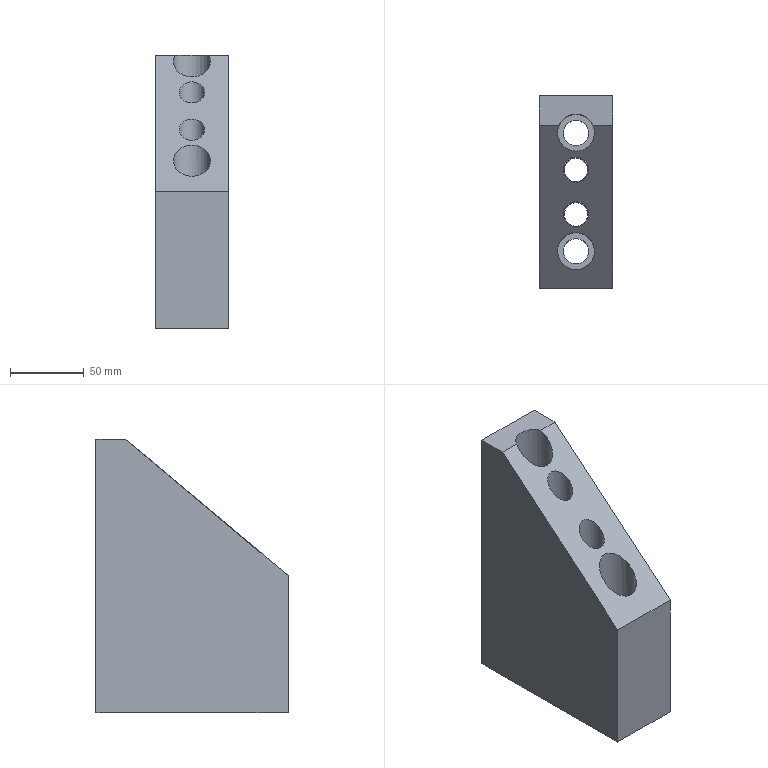Part | NX | features solid 2 | 1 solid | 19 faces | box 50 x 130 x 185 mm | volume 754988 mm3 | plane 11 | cylinder 8 | commonest cylinder face diameters 17 x4 16 x2 25 x2
STEP:
#1=CARTESIAN_POINT('',(-210.,-307.5,5.));
#2=VERTEX_POINT('',#1);
#3=CARTESIAN_POINT('',(-210.,-307.5,-150.));
#4=VERTEX_POINT('',#3);
#5=CARTESIAN_POINT('',(-210.,-307.5,-150.));
#6=DIRECTION('',(0.,0.,1.));
#7=VECTOR('',#6,1000.);
#8=LINE('',#5,#7);
#9=EDGE_CURVE('',#2,#4,#8,.F.);
#10=ORIENTED_EDGE('',*,*,#9,.T.);
#11=ORIENTED_EDGE('',*,*,#9,.F.);
#12=CARTESIAN_POINT('',(-210.,-295.,5.));
#13=VERTEX_POINT('',#12);
#14=CARTESIAN_POINT('',(-210.,-295.,5.));
#15=DIRECTION('',(0.,1.,0.));
#16=VECTOR('',#15,1000.);
#17=LINE('',#14,#16);
#18=EDGE_CURVE('',#13,#2,#17,.F.);
#19=ORIENTED_EDGE('',*,*,#18,.F.);
#20=CARTESIAN_POINT('',(-210.,-295.,-180.));
#21=VERTEX_POINT('',#20);
#22=CARTESIAN_POINT('',(-210.,-295.,5.));
#23=DIRECTION('',(0.,0.,1.));
#24=VECTOR('',#23,1000.);
#25=LINE('',#22,#24);
#26=EDGE_CURVE('',#13,#21,#25,.F.);
#27=ORIENTED_EDGE('',*,*,#26,.T.);
#28=CARTESIAN_POINT('',(-210.,-303.5,-180.));
#29=VERTEX_POINT('',#28);
#30=CARTESIAN_POINT('',(-210.,-275.,-180.));
#31=DIRECTION('',(0.,1.,0.));
#32=VECTOR('',#31,1000.);
#33=LINE('',#30,#32);
#34=EDGE_CURVE('',#29,#21,#33,.T.);
#35=ORIENTED_EDGE('',*,*,#34,.F.);
#36=CARTESIAN_POINT('',(-210.,-303.5,-150.));
#37=VERTEX_POINT('',#36);
#38=CARTESIAN_POINT('',(-210.,-303.5,-210.));
#39=DIRECTION('',(0.,0.,1.));
#40=VECTOR('',#39,1000.);
#41=LINE('',#38,#40);
#42=EDGE_CURVE('',#37,#29,#41,.F.);
#43=ORIENTED_EDGE('',*,*,#42,.F.);
#44=ORIENTED_EDGE('',*,*,#42,.T.);
#45=CARTESIAN_POINT('',(-210.,-425.,-180.));
#46=VERTEX_POINT('',#45);
#47=CARTESIAN_POINT('',(-210.,-275.,-180.));
#48=DIRECTION('',(0.,1.,0.));
#49=VECTOR('',#48,1000.);
#50=LINE('',#47,#49);
#51=EDGE_CURVE('',#46,#29,#50,.T.);
#52=ORIENTED_EDGE('',*,*,#51,.F.);
#53=CARTESIAN_POINT('',(-210.,-425.,-87.301));
#54=VERTEX_POINT('',#53);
#55=CARTESIAN_POINT('',(-210.,-425.,-120.405));
#56=DIRECTION('',(0.,0.,1.));
#57=VECTOR('',#56,1000.);
#58=LINE('',#55,#57);
#59=EDGE_CURVE('',#46,#54,#58,.T.);
#60=ORIENTED_EDGE('',*,*,#59,.T.);
#61=CARTESIAN_POINT('',(-210.,-315.,5.));
#62=VERTEX_POINT('',#61);
#63=CARTESIAN_POINT('',(-210.,-291.527,24.696));
#64=DIRECTION('',(0.,0.766,0.6428));
#65=VECTOR('',#64,1000.);
#66=LINE('',#63,#65);
#67=EDGE_CURVE('',#62,#54,#66,.F.);
#68=ORIENTED_EDGE('',*,*,#67,.F.);
#69=CARTESIAN_POINT('',(-210.,-275.,5.));
#70=DIRECTION('',(0.,-1.,0.));
#71=VECTOR('',#70,1000.);
#72=LINE('',#69,#71);
#73=EDGE_CURVE('',#2,#62,#72,.T.);
#74=ORIENTED_EDGE('',*,*,#73,.F.);
#75=EDGE_LOOP('',(#10,#11,#19,#27,#35,#43,#44,#52,#60,#68,#74));
#76=FACE_BOUND('',#75,.T.);
#77=CARTESIAN_POINT('',(-210.,-275.,5.));
#78=DIRECTION('',(-1.,0.,0.));
#79=DIRECTION('',(0.,0.,-1.));
#80=AXIS2_PLACEMENT_3D('',#77,#78,#79);
#81=PLANE('',#80);
#82=ADVANCED_FACE('',(#76),#81,.T.);
#83=CARTESIAN_POINT('',(-193.,-375.,-180.));
#84=VERTEX_POINT('',#83);
#85=CARTESIAN_POINT('',(-185.,-375.,-180.));
#86=DIRECTION('',(0.,0.,-1.));
#87=DIRECTION('',(-1.,0.,0.));
#88=AXIS2_PLACEMENT_3D('',#85,#86,#87);
#89=CIRCLE('',#88,8.);
#90=EDGE_CURVE('',#84,#84,#89,.F.);
#91=ORIENTED_EDGE('',*,*,#90,.T.);
#92=EDGE_LOOP('',(#91));
#93=FACE_BOUND('',#92,.T.);
#94=CARTESIAN_POINT('',(-193.,-345.,-180.));
#95=VERTEX_POINT('',#94);
#96=CARTESIAN_POINT('',(-185.,-345.,-180.));
#97=DIRECTION('',(0.,0.,-1.));
#98=DIRECTION('',(-1.,0.,0.));
#99=AXIS2_PLACEMENT_3D('',#96,#97,#98);
#100=CIRCLE('',#99,8.);
#101=EDGE_CURVE('',#95,#95,#100,.F.);
#102=ORIENTED_EDGE('',*,*,#101,.T.);
#103=EDGE_LOOP('',(#102));
#104=FACE_BOUND('',#103,.T.);
#105=CARTESIAN_POINT('',(-193.5,-400.,-180.));
#106=VERTEX_POINT('',#105);
#107=CARTESIAN_POINT('',(-185.,-400.,-180.));
#108=DIRECTION('',(0.,0.,-1.));
#109=DIRECTION('',(-1.,0.,0.));
#110=AXIS2_PLACEMENT_3D('',#107,#108,#109);
#111=CIRCLE('',#110,8.5);
#112=EDGE_CURVE('',#106,#106,#111,.F.);
#113=ORIENTED_EDGE('',*,*,#112,.T.);
#114=EDGE_LOOP('',(#113));
#115=FACE_BOUND('',#114,.T.);
#116=CARTESIAN_POINT('',(-193.5,-320.,-180.));
#117=VERTEX_POINT('',#116);
#118=CARTESIAN_POINT('',(-185.,-320.,-180.));
#119=DIRECTION('',(0.,0.,-1.));
#120=DIRECTION('',(-1.,0.,0.));
#121=AXIS2_PLACEMENT_3D('',#118,#119,#120);
#122=CIRCLE('',#121,8.5);
#123=EDGE_CURVE('',#117,#117,#122,.F.);
#124=ORIENTED_EDGE('',*,*,#123,.T.);
#125=EDGE_LOOP('',(#124));
#126=FACE_BOUND('',#125,.T.);
#127=ORIENTED_EDGE('',*,*,#51,.T.);
#128=ORIENTED_EDGE('',*,*,#34,.T.);
#129=CARTESIAN_POINT('',(-160.,-295.,-180.));
#130=VERTEX_POINT('',#129);
#131=CARTESIAN_POINT('',(-205.,-295.,-180.));
#132=DIRECTION('',(1.,0.,0.));
#133=VECTOR('',#132,1000.);
#134=LINE('',#131,#133);
#135=EDGE_CURVE('',#130,#21,#134,.F.);
#136=ORIENTED_EDGE('',*,*,#135,.F.);
#137=CARTESIAN_POINT('',(-160.,-425.,-180.));
#138=VERTEX_POINT('',#137);
#139=CARTESIAN_POINT('',(-160.,-275.,-180.));
#140=DIRECTION('',(0.,-1.,0.));
#141=VECTOR('',#140,1000.);
#142=LINE('',#139,#141);
#143=EDGE_CURVE('',#138,#130,#142,.F.);
#144=ORIENTED_EDGE('',*,*,#143,.F.);
#145=CARTESIAN_POINT('',(-205.,-425.,-180.));
#146=DIRECTION('',(-1.,0.,0.));
#147=VECTOR('',#146,1000.);
#148=LINE('',#145,#147);
#149=EDGE_CURVE('',#138,#46,#148,.T.);
#150=ORIENTED_EDGE('',*,*,#149,.T.);
#151=EDGE_LOOP('',(#127,#128,#136,#144,#150));
#152=FACE_BOUND('',#151,.T.);
#153=CARTESIAN_POINT('',(-205.,-275.,-180.));
#154=DIRECTION('',(0.,0.,-1.));
#155=DIRECTION('',(1.,0.,0.));
#156=AXIS2_PLACEMENT_3D('',#153,#154,#155);
#157=PLANE('',#156);
#158=ADVANCED_FACE('',(#93,#104,#115,#126,#152),#157,.T.);
#159=CARTESIAN_POINT('',(-160.,-295.,5.));
#160=VERTEX_POINT('',#159);
#161=CARTESIAN_POINT('',(-160.,-295.,5.));
#162=DIRECTION('',(0.,0.,-1.));
#163=VECTOR('',#162,1000.);
#164=LINE('',#161,#163);
#165=EDGE_CURVE('',#160,#130,#164,.T.);
#166=ORIENTED_EDGE('',*,*,#165,.F.);
#167=CARTESIAN_POINT('',(-160.,-315.,5.));
#168=VERTEX_POINT('',#167);
#169=CARTESIAN_POINT('',(-160.,-295.,5.));
#170=DIRECTION('',(0.,1.,0.));
#171=VECTOR('',#170,1000.);
#172=LINE('',#169,#171);
#173=EDGE_CURVE('',#168,#160,#172,.T.);
#174=ORIENTED_EDGE('',*,*,#173,.F.);
#175=CARTESIAN_POINT('',(-160.,-425.,-87.301));
#176=VERTEX_POINT('',#175);
#177=CARTESIAN_POINT('',(-160.,-330.716,-8.188));
#178=DIRECTION('',(0.,-0.766,-0.6428));
#179=VECTOR('',#178,1000.);
#180=LINE('',#177,#179);
#181=EDGE_CURVE('',#168,#176,#180,.T.);
#182=ORIENTED_EDGE('',*,*,#181,.T.);
#183=CARTESIAN_POINT('',(-160.,-425.,-120.405));
#184=DIRECTION('',(0.,0.,1.));
#185=VECTOR('',#184,1000.);
#186=LINE('',#183,#185);
#187=EDGE_CURVE('',#176,#138,#186,.F.);
#188=ORIENTED_EDGE('',*,*,#187,.T.);
#189=ORIENTED_EDGE('',*,*,#143,.T.);
#190=EDGE_LOOP('',(#166,#174,#182,#188,#189));
#191=FACE_BOUND('',#190,.T.);
#192=CARTESIAN_POINT('',(-160.,-275.,5.));
#193=DIRECTION('',(-1.,0.,0.));
#194=DIRECTION('',(0.,0.,-1.));
#195=AXIS2_PLACEMENT_3D('',#192,#193,#194);
#196=PLANE('',#195);
#197=ADVANCED_FACE('',(#191),#196,.F.);
#198=CARTESIAN_POINT('',(-196.456,-315.,5.));
#199=VERTEX_POINT('',#198);
#200=CARTESIAN_POINT('',(-205.,-315.,5.));
#201=DIRECTION('',(1.,0.,0.));
#202=VECTOR('',#201,1000.);
#203=LINE('',#200,#202);
#204=EDGE_CURVE('',#62,#199,#203,.T.);
#205=ORIENTED_EDGE('',*,*,#204,.T.);
#206=CARTESIAN_POINT('',(-173.544,-315.,5.));
#207=VERTEX_POINT('',#206);
#208=CARTESIAN_POINT('',(-185.,-320.,5.));
#209=DIRECTION('',(0.,0.,-1.));
#210=DIRECTION('',(-1.,0.,0.));
#211=AXIS2_PLACEMENT_3D('',#208,#209,#210);
#212=CIRCLE('',#211,12.5);
#213=EDGE_CURVE('',#199,#207,#212,.T.);
#214=ORIENTED_EDGE('',*,*,#213,.T.);
#215=CARTESIAN_POINT('',(-205.,-315.,5.));
#216=DIRECTION('',(1.,0.,0.));
#217=VECTOR('',#216,1000.);
#218=LINE('',#215,#217);
#219=EDGE_CURVE('',#207,#168,#218,.T.);
#220=ORIENTED_EDGE('',*,*,#219,.T.);
#221=ORIENTED_EDGE('',*,*,#173,.T.);
#222=CARTESIAN_POINT('',(-110.,-295.,5.));
#223=DIRECTION('',(1.,0.,0.));
#224=VECTOR('',#223,1000.);
#225=LINE('',#222,#224);
#226=EDGE_CURVE('',#13,#160,#225,.T.);
#227=ORIENTED_EDGE('',*,*,#226,.F.);
#228=ORIENTED_EDGE('',*,*,#18,.T.);
#229=ORIENTED_EDGE('',*,*,#73,.T.);
#230=EDGE_LOOP('',(#205,#214,#220,#221,#227,#228,#229));
#231=FACE_BOUND('',#230,.T.);
#232=CARTESIAN_POINT('',(-110.,-295.,5.));
#233=DIRECTION('',(0.,0.,-1.));
#234=DIRECTION('',(-1.,0.,0.));
#235=AXIS2_PLACEMENT_3D('',#232,#233,#234);
#236=PLANE('',#235);
#237=ADVANCED_FACE('',(#231),#236,.F.);
#238=CARTESIAN_POINT('',(-185.,-366.5,-38.214));
#239=VERTEX_POINT('',#238);
#240=CARTESIAN_POINT('',(-185.,-375.,-45.346));
#241=DIRECTION('',(0.,-0.6428,0.766));
#242=DIRECTION('',(0.,0.766,0.6428));
#243=AXIS2_PLACEMENT_3D('',#240,#241,#242);
#244=ELLIPSE('',#243,11.096,8.5);
#245=EDGE_CURVE('',#239,#239,#244,.T.);
#246=ORIENTED_EDGE('',*,*,#245,.F.);
#247=EDGE_LOOP('',(#246));
#248=FACE_BOUND('',#247,.T.);
#249=CARTESIAN_POINT('',(-185.,-336.5,-13.041));
#250=VERTEX_POINT('',#249);
#251=CARTESIAN_POINT('',(-185.,-345.,-20.173));
#252=DIRECTION('',(0.,-0.6428,0.766));
#253=DIRECTION('',(0.,0.766,0.6428));
#254=AXIS2_PLACEMENT_3D('',#251,#252,#253);
#255=ELLIPSE('',#254,11.096,8.5);
#256=EDGE_CURVE('',#250,#250,#255,.T.);
#257=ORIENTED_EDGE('',*,*,#256,.F.);
#258=EDGE_LOOP('',(#257));
#259=FACE_BOUND('',#258,.T.);
#260=CARTESIAN_POINT('',(-185.,-387.5,-55.835));
#261=VERTEX_POINT('',#260);
#262=CARTESIAN_POINT('',(-185.,-400.,-66.323));
#263=DIRECTION('',(0.,-0.6428,0.766));
#264=DIRECTION('',(0.,0.766,0.6428));
#265=AXIS2_PLACEMENT_3D('',#262,#263,#264);
#266=ELLIPSE('',#265,16.318,12.5);
#267=EDGE_CURVE('',#261,#261,#266,.T.);
#268=ORIENTED_EDGE('',*,*,#267,.F.);
#269=EDGE_LOOP('',(#268));
#270=FACE_BOUND('',#269,.T.);
#271=CARTESIAN_POINT('',(-185.,-320.,0.8045));
#272=DIRECTION('',(0.,-0.6428,0.766));
#273=DIRECTION('',(0.,0.766,0.6428));
#274=AXIS2_PLACEMENT_3D('',#271,#272,#273);
#275=ELLIPSE('',#274,16.318,12.5);
#276=EDGE_CURVE('',#199,#207,#275,.T.);
#277=ORIENTED_EDGE('',*,*,#276,.F.);
#278=ORIENTED_EDGE('',*,*,#204,.F.);
#279=ORIENTED_EDGE('',*,*,#67,.T.);
#280=CARTESIAN_POINT('',(-205.,-425.,-87.301));
#281=DIRECTION('',(-1.,0.,0.));
#282=VECTOR('',#281,1000.);
#283=LINE('',#280,#282);
#284=EDGE_CURVE('',#54,#176,#283,.F.);
#285=ORIENTED_EDGE('',*,*,#284,.T.);
#286=ORIENTED_EDGE('',*,*,#181,.F.);
#287=ORIENTED_EDGE('',*,*,#219,.F.);
#288=EDGE_LOOP('',(#277,#278,#279,#285,#286,#287));
#289=FACE_BOUND('',#288,.T.);
#290=CARTESIAN_POINT('',(-205.,-330.716,-8.188));
#291=DIRECTION('',(0.,-0.6428,0.766));
#292=DIRECTION('',(0.,-0.766,-0.6428));
#293=AXIS2_PLACEMENT_3D('',#290,#291,#292);
#294=PLANE('',#293);
#295=ADVANCED_FACE('',(#248,#259,#270,#289),#294,.T.);
#296=ORIENTED_EDGE('',*,*,#59,.F.);
#297=ORIENTED_EDGE('',*,*,#149,.F.);
#298=ORIENTED_EDGE('',*,*,#187,.F.);
#299=ORIENTED_EDGE('',*,*,#284,.F.);
#300=EDGE_LOOP('',(#296,#297,#298,#299));
#301=FACE_BOUND('',#300,.T.);
#302=CARTESIAN_POINT('',(-205.,-425.,-120.405));
#303=DIRECTION('',(0.,1.,0.));
#304=DIRECTION('',(0.,0.,1.));
#305=AXIS2_PLACEMENT_3D('',#302,#303,#304);
#306=PLANE('',#305);
#307=ADVANCED_FACE('',(#301),#306,.F.);
#308=ORIENTED_EDGE('',*,*,#135,.T.);
#309=ORIENTED_EDGE('',*,*,#26,.F.);
#310=ORIENTED_EDGE('',*,*,#226,.T.);
#311=ORIENTED_EDGE('',*,*,#165,.T.);
#312=EDGE_LOOP('',(#308,#309,#310,#311));
#313=FACE_BOUND('',#312,.T.);
#314=CARTESIAN_POINT('',(-110.,-295.,5.));
#315=DIRECTION('',(0.,1.,0.));
#316=DIRECTION('',(0.,0.,1.));
#317=AXIS2_PLACEMENT_3D('',#314,#315,#316);
#318=PLANE('',#317);
#319=ADVANCED_FACE('',(#313),#318,.T.);
#320=CARTESIAN_POINT('',(-193.5,-320.,-150.));
#321=VERTEX_POINT('',#320);
#322=CARTESIAN_POINT('',(-185.,-320.,-150.));
#323=DIRECTION('',(0.,0.,-1.));
#324=DIRECTION('',(-1.,0.,0.));
#325=AXIS2_PLACEMENT_3D('',#322,#323,#324);
#326=CIRCLE('',#325,8.5);
#327=EDGE_CURVE('',#321,#321,#326,.F.);
#328=ORIENTED_EDGE('',*,*,#327,.T.);
#329=EDGE_LOOP('',(#328));
#330=FACE_BOUND('',#329,.T.);
#331=ORIENTED_EDGE('',*,*,#123,.F.);
#332=EDGE_LOOP('',(#331));
#333=FACE_BOUND('',#332,.T.);
#334=CARTESIAN_POINT('',(-185.,-320.,-210.));
#335=DIRECTION('',(0.,0.,1.));
#336=DIRECTION('',(1.,0.,0.));
#337=AXIS2_PLACEMENT_3D('',#334,#335,#336);
#338=CYLINDRICAL_SURFACE('',#337,8.5);
#339=ADVANCED_FACE('',(#330,#333),#338,.F.);
#340=CARTESIAN_POINT('',(-172.5,-320.,-150.));
#341=VERTEX_POINT('',#340);
#342=CARTESIAN_POINT('',(-185.,-320.,-150.));
#343=DIRECTION('',(0.,0.,1.));
#344=DIRECTION('',(1.,0.,0.));
#345=AXIS2_PLACEMENT_3D('',#342,#343,#344);
#346=CIRCLE('',#345,12.5);
#347=EDGE_CURVE('',#341,#341,#346,.T.);
#348=ORIENTED_EDGE('',*,*,#347,.F.);
#349=EDGE_LOOP('',(#348));
#350=FACE_BOUND('',#349,.T.);
#351=ORIENTED_EDGE('',*,*,#276,.T.);
#352=ORIENTED_EDGE('',*,*,#213,.F.);
#353=EDGE_LOOP('',(#351,#352));
#354=FACE_BOUND('',#353,.T.);
#355=CARTESIAN_POINT('',(-185.,-320.,-150.));
#356=DIRECTION('',(0.,0.,1.));
#357=DIRECTION('',(1.,0.,0.));
#358=AXIS2_PLACEMENT_3D('',#355,#356,#357);
#359=CYLINDRICAL_SURFACE('',#358,12.5);
#360=ADVANCED_FACE('',(#350,#354),#359,.F.);
#361=ORIENTED_EDGE('',*,*,#327,.F.);
#362=EDGE_LOOP('',(#361));
#363=FACE_BOUND('',#362,.T.);
#364=ORIENTED_EDGE('',*,*,#347,.T.);
#365=EDGE_LOOP('',(#364));
#366=FACE_BOUND('',#365,.T.);
#367=CARTESIAN_POINT('',(-185.,-320.,-150.));
#368=DIRECTION('',(0.,0.,-1.));
#369=DIRECTION('',(-1.,0.,0.));
#370=AXIS2_PLACEMENT_3D('',#367,#368,#369);
#371=PLANE('',#370);
#372=ADVANCED_FACE('',(#363,#366),#371,.F.);
#373=CARTESIAN_POINT('',(-193.5,-400.,-150.));
#374=VERTEX_POINT('',#373);
#375=CARTESIAN_POINT('',(-185.,-400.,-150.));
#376=DIRECTION('',(0.,0.,-1.));
#377=DIRECTION('',(-1.,0.,0.));
#378=AXIS2_PLACEMENT_3D('',#375,#376,#377);
#379=CIRCLE('',#378,8.5);
#380=EDGE_CURVE('',#374,#374,#379,.F.);
#381=ORIENTED_EDGE('',*,*,#380,.T.);
#382=EDGE_LOOP('',(#381));
#383=FACE_BOUND('',#382,.T.);
#384=ORIENTED_EDGE('',*,*,#112,.F.);
#385=EDGE_LOOP('',(#384));
#386=FACE_BOUND('',#385,.T.);
#387=CARTESIAN_POINT('',(-185.,-400.,-210.));
#388=DIRECTION('',(0.,0.,1.));
#389=DIRECTION('',(1.,0.,0.));
#390=AXIS2_PLACEMENT_3D('',#387,#388,#389);
#391=CYLINDRICAL_SURFACE('',#390,8.5);
#392=ADVANCED_FACE('',(#383,#386),#391,.F.);
#393=ORIENTED_EDGE('',*,*,#380,.F.);
#394=EDGE_LOOP('',(#393));
#395=FACE_BOUND('',#394,.T.);
#396=CARTESIAN_POINT('',(-172.5,-400.,-150.));
#397=VERTEX_POINT('',#396);
#398=CARTESIAN_POINT('',(-185.,-400.,-150.));
#399=DIRECTION('',(0.,0.,1.));
#400=DIRECTION('',(1.,0.,0.));
#401=AXIS2_PLACEMENT_3D('',#398,#399,#400);
#402=CIRCLE('',#401,12.5);
#403=EDGE_CURVE('',#397,#397,#402,.T.);
#404=ORIENTED_EDGE('',*,*,#403,.T.);
#405=EDGE_LOOP('',(#404));
#406=FACE_BOUND('',#405,.T.);
#407=CARTESIAN_POINT('',(-185.,-400.,-150.));
#408=DIRECTION('',(0.,0.,-1.));
#409=DIRECTION('',(-1.,0.,0.));
#410=AXIS2_PLACEMENT_3D('',#407,#408,#409);
#411=PLANE('',#410);
#412=ADVANCED_FACE('',(#395,#406),#411,.F.);
#413=ORIENTED_EDGE('',*,*,#267,.T.);
#414=EDGE_LOOP('',(#413));
#415=FACE_BOUND('',#414,.T.);
#416=ORIENTED_EDGE('',*,*,#403,.F.);
#417=EDGE_LOOP('',(#416));
#418=FACE_BOUND('',#417,.T.);
#419=CARTESIAN_POINT('',(-185.,-400.,-150.));
#420=DIRECTION('',(0.,0.,1.));
#421=DIRECTION('',(1.,0.,0.));
#422=AXIS2_PLACEMENT_3D('',#419,#420,#421);
#423=CYLINDRICAL_SURFACE('',#422,12.5);
#424=ADVANCED_FACE('',(#415,#418),#423,.F.);
#425=CARTESIAN_POINT('',(-185.,-337.,-150.));
#426=VERTEX_POINT('',#425);
#427=CARTESIAN_POINT('',(-185.,-345.,-150.));
#428=DIRECTION('',(0.,0.,-1.));
#429=DIRECTION('',(0.,1.,0.));
#430=AXIS2_PLACEMENT_3D('',#427,#428,#429);
#431=CIRCLE('',#430,8.);
#432=EDGE_CURVE('',#426,#426,#431,.F.);
#433=ORIENTED_EDGE('',*,*,#432,.T.);
#434=EDGE_LOOP('',(#433));
#435=FACE_BOUND('',#434,.T.);
#436=ORIENTED_EDGE('',*,*,#101,.F.);
#437=EDGE_LOOP('',(#436));
#438=FACE_BOUND('',#437,.T.);
#439=CARTESIAN_POINT('',(-185.,-345.,-210.));
#440=DIRECTION('',(0.,0.,1.));
#441=DIRECTION('',(0.,-1.,0.));
#442=AXIS2_PLACEMENT_3D('',#439,#440,#441);
#443=CYLINDRICAL_SURFACE('',#442,8.);
#444=ADVANCED_FACE('',(#435,#438),#443,.F.);
#445=ORIENTED_EDGE('',*,*,#432,.F.);
#446=EDGE_LOOP('',(#445));
#447=FACE_BOUND('',#446,.T.);
#448=CARTESIAN_POINT('',(-185.,-353.5,-150.));
#449=VERTEX_POINT('',#448);
#450=CARTESIAN_POINT('',(-185.,-345.,-150.));
#451=DIRECTION('',(0.,0.,1.));
#452=DIRECTION('',(0.,-1.,0.));
#453=AXIS2_PLACEMENT_3D('',#450,#451,#452);
#454=CIRCLE('',#453,8.5);
#455=EDGE_CURVE('',#449,#449,#454,.T.);
#456=ORIENTED_EDGE('',*,*,#455,.T.);
#457=EDGE_LOOP('',(#456));
#458=FACE_BOUND('',#457,.T.);
#459=CARTESIAN_POINT('',(-185.,-345.,-150.));
#460=DIRECTION('',(0.,0.,-1.));
#461=DIRECTION('',(0.,1.,0.));
#462=AXIS2_PLACEMENT_3D('',#459,#460,#461);
#463=PLANE('',#462);
#464=ADVANCED_FACE('',(#447,#458),#463,.F.);
#465=ORIENTED_EDGE('',*,*,#256,.T.);
#466=EDGE_LOOP('',(#465));
#467=FACE_BOUND('',#466,.T.);
#468=ORIENTED_EDGE('',*,*,#455,.F.);
#469=EDGE_LOOP('',(#468));
#470=FACE_BOUND('',#469,.T.);
#471=CARTESIAN_POINT('',(-185.,-345.,-150.));
#472=DIRECTION('',(0.,0.,1.));
#473=DIRECTION('',(0.,-1.,0.));
#474=AXIS2_PLACEMENT_3D('',#471,#472,#473);
#475=CYLINDRICAL_SURFACE('',#474,8.5);
#476=ADVANCED_FACE('',(#467,#470),#475,.F.);
#477=CARTESIAN_POINT('',(-193.,-375.,-150.));
#478=VERTEX_POINT('',#477);
#479=CARTESIAN_POINT('',(-185.,-375.,-150.));
#480=DIRECTION('',(0.,0.,-1.));
#481=DIRECTION('',(-1.,0.,0.));
#482=AXIS2_PLACEMENT_3D('',#479,#480,#481);
#483=CIRCLE('',#482,8.);
#484=EDGE_CURVE('',#478,#478,#483,.F.);
#485=ORIENTED_EDGE('',*,*,#484,.T.);
#486=EDGE_LOOP('',(#485));
#487=FACE_BOUND('',#486,.T.);
#488=ORIENTED_EDGE('',*,*,#90,.F.);
#489=EDGE_LOOP('',(#488));
#490=FACE_BOUND('',#489,.T.);
#491=CARTESIAN_POINT('',(-185.,-375.,-210.));
#492=DIRECTION('',(0.,0.,1.));
#493=DIRECTION('',(1.,0.,0.));
#494=AXIS2_PLACEMENT_3D('',#491,#492,#493);
#495=CYLINDRICAL_SURFACE('',#494,8.);
#496=ADVANCED_FACE('',(#487,#490),#495,.F.);
#497=ORIENTED_EDGE('',*,*,#484,.F.);
#498=EDGE_LOOP('',(#497));
#499=FACE_BOUND('',#498,.T.);
#500=CARTESIAN_POINT('',(-176.5,-375.,-150.));
#501=VERTEX_POINT('',#500);
#502=CARTESIAN_POINT('',(-185.,-375.,-150.));
#503=DIRECTION('',(0.,0.,1.));
#504=DIRECTION('',(1.,0.,0.));
#505=AXIS2_PLACEMENT_3D('',#502,#503,#504);
#506=CIRCLE('',#505,8.5);
#507=EDGE_CURVE('',#501,#501,#506,.T.);
#508=ORIENTED_EDGE('',*,*,#507,.T.);
#509=EDGE_LOOP('',(#508));
#510=FACE_BOUND('',#509,.T.);
#511=CARTESIAN_POINT('',(-185.,-375.,-150.));
#512=DIRECTION('',(0.,0.,-1.));
#513=DIRECTION('',(-1.,0.,0.));
#514=AXIS2_PLACEMENT_3D('',#511,#512,#513);
#515=PLANE('',#514);
#516=ADVANCED_FACE('',(#499,#510),#515,.F.);
#517=ORIENTED_EDGE('',*,*,#245,.T.);
#518=EDGE_LOOP('',(#517));
#519=FACE_BOUND('',#518,.T.);
#520=ORIENTED_EDGE('',*,*,#507,.F.);
#521=EDGE_LOOP('',(#520));
#522=FACE_BOUND('',#521,.T.);
#523=CARTESIAN_POINT('',(-185.,-375.,-150.));
#524=DIRECTION('',(0.,0.,1.));
#525=DIRECTION('',(1.,0.,0.));
#526=AXIS2_PLACEMENT_3D('',#523,#524,#525);
#527=CYLINDRICAL_SURFACE('',#526,8.5);
#528=ADVANCED_FACE('',(#519,#522),#527,.F.);
#529=CLOSED_SHELL('',(#82,#158,#197,#237,#295,#307,#319,#339,#360,#372,#392,#412,#424,#444,#464,#476,#496,#516,#528));
#530=MANIFOLD_SOLID_BREP('',#529);
#531=(LENGTH_UNIT()NAMED_UNIT(*)SI_UNIT(.MILLI.,.METRE.));
#532=UNCERTAINTY_MEASURE_WITH_UNIT(LENGTH_MEASURE(0.00001),#531,'','');
#533=(NAMED_UNIT(*)PLANE_ANGLE_UNIT()SI_UNIT($,.RADIAN.));
#534=(NAMED_UNIT(*)SI_UNIT($,.STERADIAN.)SOLID_ANGLE_UNIT());
#535=(GEOMETRIC_REPRESENTATION_CONTEXT(3)GLOBAL_UNCERTAINTY_ASSIGNED_CONTEXT((#532))GLOBAL_UNIT_ASSIGNED_CONTEXT((#531,#533,#534))REPRESENTATION_CONTEXT('',''));
#536=ADVANCED_BREP_SHAPE_REPRESENTATION('',(#530),#535);